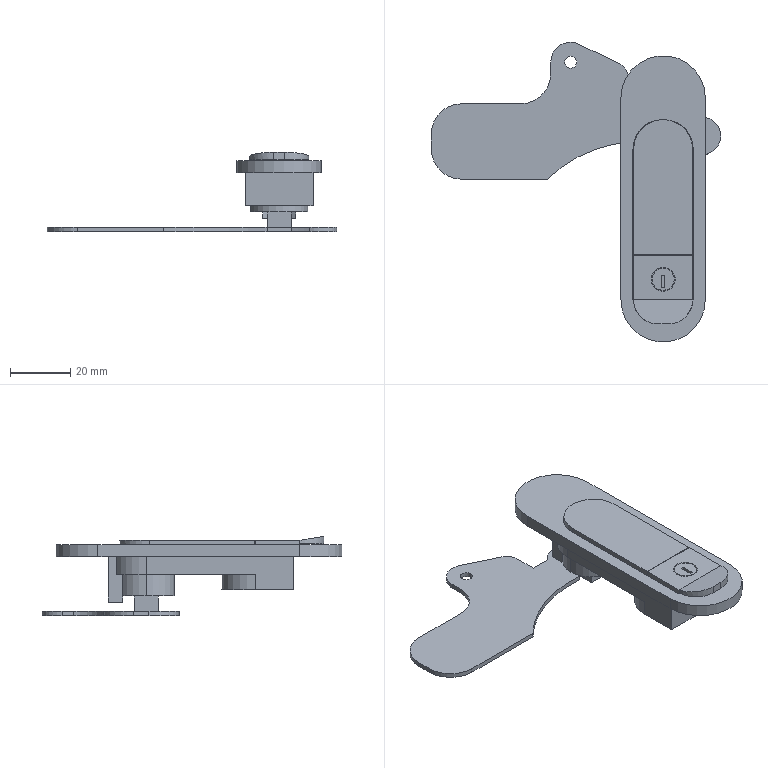Part | STEP file | HBX303 | 2 solids | 122 faces | box 96.026 x 99.517 x 26.27 mm | volume 23876 mm3 | plane 80 | cylinder 42 | commonest cylinder face diameters 4 x6 20 x5 19 x4 10 x3 22.5 x3 7.322 x2